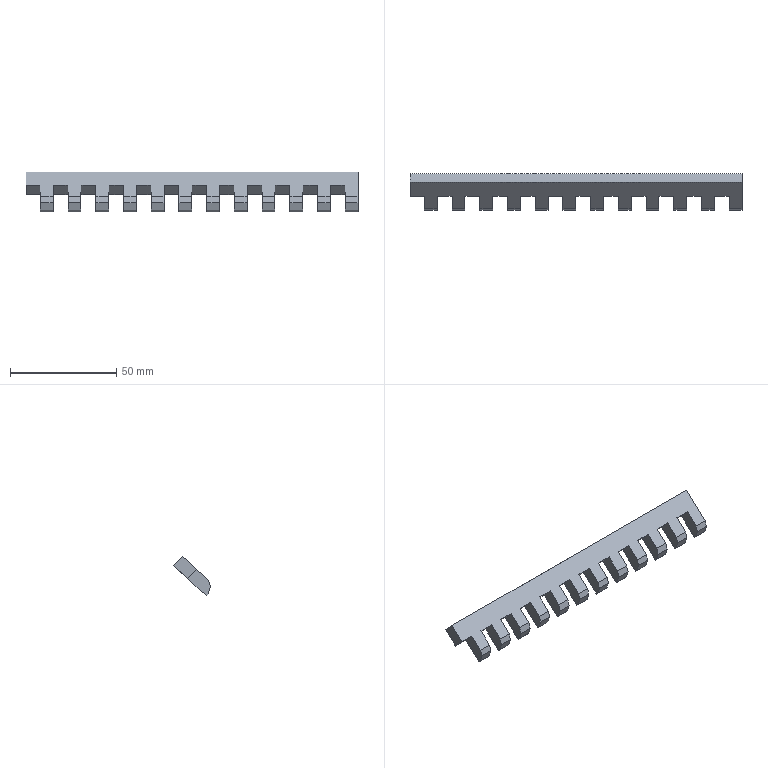Part | NX | 1 solid | 76 faces | box 156 x 17.318 x 18.649 mm | volume 12986 mm3 | plane 75 | cylinder 1 | commonest cylinder face diameters 42 x1